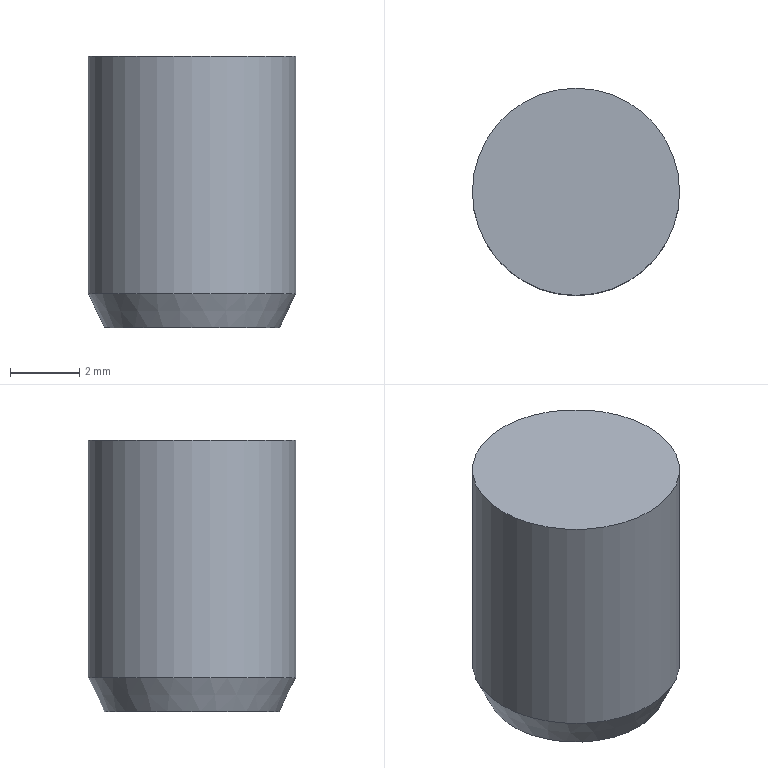Part | NX | features 9416K301(body) 2 | 1 solid | 4 faces | box 6 x 6 x 7.874 mm | volume 218.54 mm3 | plane 2 | cylinder 1 | cone 1 | commonest cylinder face diameters 6 x1
STEP:
#1=CARTESIAN_POINT('',(0.,-3.,-74.93));
#2=VERTEX_POINT('',#1);
#3=CARTESIAN_POINT('',(0.,0.,-74.93));
#4=DIRECTION('',(0.,0.,1.));
#5=DIRECTION('',(0.,-1.,0.));
#6=AXIS2_PLACEMENT_3D('',#3,#4,#5);
#7=CIRCLE('',#6,3.);
#8=EDGE_CURVE('',#2,#2,#7,.T.);
#9=ORIENTED_EDGE('',*,*,#8,.F.);
#10=EDGE_LOOP('',(#9));
#11=FACE_BOUND('',#10,.T.);
#12=CARTESIAN_POINT('',(3.,0.,-81.813));
#13=VERTEX_POINT('',#12);
#14=CARTESIAN_POINT('',(0.,0.,-81.813));
#15=DIRECTION('',(0.,0.,1.));
#16=DIRECTION('',(1.,0.,0.));
#17=AXIS2_PLACEMENT_3D('',#14,#15,#16);
#18=CIRCLE('',#17,3.);
#19=EDGE_CURVE('',#13,#13,#18,.T.);
#20=ORIENTED_EDGE('',*,*,#19,.T.);
#21=EDGE_LOOP('',(#20));
#22=FACE_BOUND('',#21,.T.);
#23=CARTESIAN_POINT('',(0.,0.,-74.93));
#24=DIRECTION('',(0.,0.,1.));
#25=DIRECTION('',(0.,-1.,0.));
#26=AXIS2_PLACEMENT_3D('',#23,#24,#25);
#27=CYLINDRICAL_SURFACE('',#26,3.);
#28=ADVANCED_FACE('',(#11,#22),#27,.T.);
#29=ORIENTED_EDGE('',*,*,#8,.T.);
#30=EDGE_LOOP('',(#29));
#31=FACE_BOUND('',#30,.T.);
#32=CARTESIAN_POINT('',(0.,0.,-74.93));
#33=DIRECTION('',(0.,0.,-1.));
#34=DIRECTION('',(0.,1.,0.));
#35=AXIS2_PLACEMENT_3D('',#32,#33,#34);
#36=PLANE('',#35);
#37=ADVANCED_FACE('',(#31),#36,.F.);
#38=CARTESIAN_POINT('',(2.538,0.,-82.804));
#39=VERTEX_POINT('',#38);
#40=CARTESIAN_POINT('',(0.,0.,-82.804));
#41=DIRECTION('',(0.,0.,1.));
#42=DIRECTION('',(1.,0.,0.));
#43=AXIS2_PLACEMENT_3D('',#40,#41,#42);
#44=CIRCLE('',#43,2.538);
#45=EDGE_CURVE('',#39,#39,#44,.T.);
#46=ORIENTED_EDGE('',*,*,#45,.T.);
#47=EDGE_LOOP('',(#46));
#48=FACE_BOUND('',#47,.T.);
#49=ORIENTED_EDGE('',*,*,#19,.F.);
#50=EDGE_LOOP('',(#49));
#51=FACE_BOUND('',#50,.T.);
#52=CARTESIAN_POINT('',(0.,0.,-81.813));
#53=DIRECTION('',(0.,0.,1.));
#54=DIRECTION('',(1.,0.,0.));
#55=AXIS2_PLACEMENT_3D('',#52,#53,#54);
#56=CONICAL_SURFACE('',#55,3.,0.4363);
#57=ADVANCED_FACE('',(#48,#51),#56,.T.);
#58=ORIENTED_EDGE('',*,*,#45,.F.);
#59=EDGE_LOOP('',(#58));
#60=FACE_BOUND('',#59,.T.);
#61=CARTESIAN_POINT('',(0.,3.,-82.804));
#62=DIRECTION('',(0.,0.,1.));
#63=DIRECTION('',(0.,-1.,0.));
#64=AXIS2_PLACEMENT_3D('',#61,#62,#63);
#65=PLANE('',#64);
#66=ADVANCED_FACE('',(#60),#65,.F.);
#67=CLOSED_SHELL('',(#28,#37,#57,#66));
#68=MANIFOLD_SOLID_BREP('',#67);
#69=(LENGTH_UNIT()NAMED_UNIT(*)SI_UNIT(.MILLI.,.METRE.));
#70=UNCERTAINTY_MEASURE_WITH_UNIT(LENGTH_MEASURE(0.00001),#69,'','');
#71=(NAMED_UNIT(*)PLANE_ANGLE_UNIT()SI_UNIT($,.RADIAN.));
#72=(NAMED_UNIT(*)SI_UNIT($,.STERADIAN.)SOLID_ANGLE_UNIT());
#73=(GEOMETRIC_REPRESENTATION_CONTEXT(3)GLOBAL_UNCERTAINTY_ASSIGNED_CONTEXT((#70))GLOBAL_UNIT_ASSIGNED_CONTEXT((#69,#71,#72))REPRESENTATION_CONTEXT('',''));
#74=ADVANCED_BREP_SHAPE_REPRESENTATION('',(#68),#73);